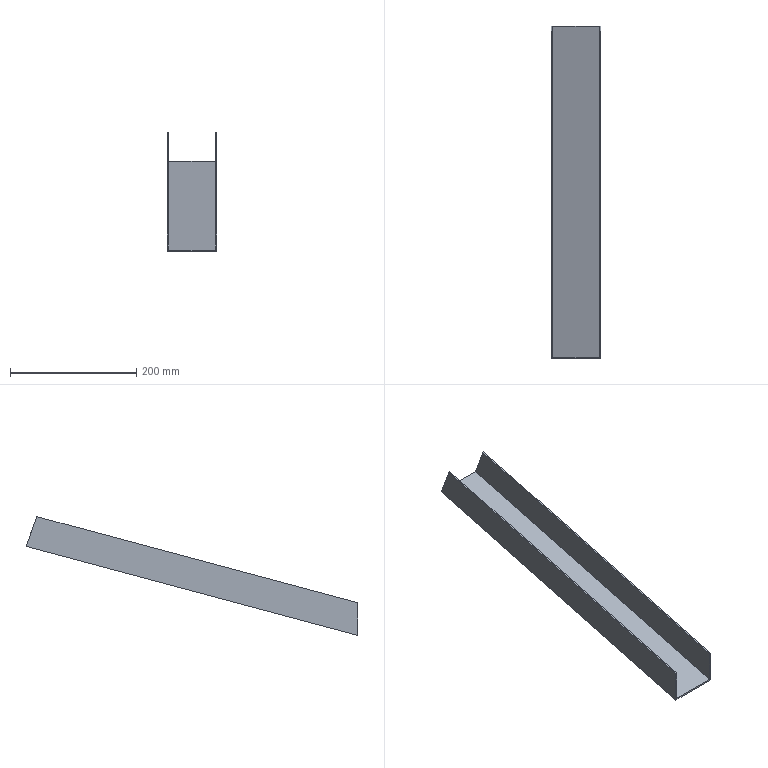Part | NX | features solid 2 | 1 solid | 10 faces | box 78 x 525 x 187.837 mm | volume 187315 mm3 | plane 9 | spline 1
STEP:
#1=CARTESIAN_POINT('',(767.,-915.,-591.646));
#2=VERTEX_POINT('',#1);
#3=CARTESIAN_POINT('',(767.,-407.166,-455.572));
#4=VERTEX_POINT('',#3);
#5=CARTESIAN_POINT('',(767.,-935.325,-597.092));
#6=DIRECTION('',(0.,0.9659,0.2588));
#7=VECTOR('',#6,1000.);
#8=LINE('',#5,#7);
#9=EDGE_CURVE('',#2,#4,#8,.T.);
#10=ORIENTED_EDGE('',*,*,#9,.T.);
#11=CARTESIAN_POINT('',(767.,-390.,-502.736));
#12=VERTEX_POINT('',#11);
#13=CARTESIAN_POINT('',(767.,-407.111,-455.724));
#14=DIRECTION('',(0.,-0.342,0.9397));
#15=VECTOR('',#14,1000.);
#16=LINE('',#13,#15);
#17=EDGE_CURVE('',#12,#4,#16,.T.);
#18=ORIENTED_EDGE('',*,*,#17,.F.);
#19=CARTESIAN_POINT('',(767.,-915.,-643.409));
#20=VERTEX_POINT('',#19);
#21=CARTESIAN_POINT('',(767.,-49.599,-411.526));
#22=DIRECTION('',(0.,0.9659,0.2588));
#23=VECTOR('',#22,1000.);
#24=LINE('',#21,#23);
#25=EDGE_CURVE('',#20,#12,#24,.T.);
#26=ORIENTED_EDGE('',*,*,#25,.F.);
#27=CARTESIAN_POINT('',(767.,-915.,-643.456));
#28=DIRECTION('',(0.,0.,-1.));
#29=VECTOR('',#28,1000.);
#30=LINE('',#27,#29);
#31=EDGE_CURVE('',#2,#20,#30,.T.);
#32=ORIENTED_EDGE('',*,*,#31,.F.);
#33=EDGE_LOOP('',(#10,#18,#26,#32));
#34=FACE_BOUND('',#33,.T.);
#35=CARTESIAN_POINT('',(767.,-922.902,-643.456));
#36=DIRECTION('',(1.,0.,0.));
#37=DIRECTION('',(0.,0.08716,0.9962));
#38=AXIS2_PLACEMENT_3D('',#35,#36,#37);
#39=PLANE('',#38);
#40=ADVANCED_FACE('',(#34),#39,.F.);
#41=CARTESIAN_POINT('',(845.,-915.,-591.646));
#42=VERTEX_POINT('',#41);
#43=CARTESIAN_POINT('',(845.,-915.,-643.409));
#44=VERTEX_POINT('',#43);
#45=CARTESIAN_POINT('',(845.,-915.,-591.646));
#46=CARTESIAN_POINT('',(845.,-915.,-608.9));
#47=CARTESIAN_POINT('',(845.,-915.,-626.155));
#48=CARTESIAN_POINT('',(845.,-915.,-643.409));
#49=B_SPLINE_CURVE_WITH_KNOTS('',3,(#45,#46,#47,#48),.UNSPECIFIED.,.F.,.F.,(4,4),(0.08523,0.137),.UNSPECIFIED.);
#50=EDGE_CURVE('',#42,#44,#49,.T.);
#51=ORIENTED_EDGE('',*,*,#50,.T.);
#52=CARTESIAN_POINT('',(845.,-390.,-502.736));
#53=VERTEX_POINT('',#52);
#54=CARTESIAN_POINT('',(845.,-49.599,-411.526));
#55=DIRECTION('',(0.,0.9659,0.2588));
#56=VECTOR('',#55,1000.);
#57=LINE('',#54,#56);
#58=EDGE_CURVE('',#44,#53,#57,.T.);
#59=ORIENTED_EDGE('',*,*,#58,.T.);
#60=CARTESIAN_POINT('',(845.,-407.166,-455.572));
#61=VERTEX_POINT('',#60);
#62=CARTESIAN_POINT('',(845.,-407.111,-455.724));
#63=DIRECTION('',(0.,-0.342,0.9397));
#64=VECTOR('',#63,1000.);
#65=LINE('',#62,#64);
#66=EDGE_CURVE('',#53,#61,#65,.T.);
#67=ORIENTED_EDGE('',*,*,#66,.T.);
#68=CARTESIAN_POINT('',(845.,-935.325,-597.092));
#69=DIRECTION('',(0.,-0.9659,-0.2588));
#70=VECTOR('',#69,1000.);
#71=LINE('',#68,#70);
#72=EDGE_CURVE('',#42,#61,#71,.F.);
#73=ORIENTED_EDGE('',*,*,#72,.F.);
#74=EDGE_LOOP('',(#51,#59,#67,#73));
#75=FACE_BOUND('',#74,.T.);
#76=CARTESIAN_POINT('',(845.,-922.902,-643.456));
#77=DIRECTION('',(1.,0.,0.));
#78=DIRECTION('',(0.,0.08716,0.9962));
#79=AXIS2_PLACEMENT_3D('',#76,#77,#78);
#80=PLANE('',#79);
#81=ADVANCED_FACE('',(#75),#80,.T.);
#82=CARTESIAN_POINT('',(843.,-390.687,-500.85));
#83=VERTEX_POINT('',#82);
#84=CARTESIAN_POINT('',(843.,-915.,-641.339));
#85=VERTEX_POINT('',#84);
#86=CARTESIAN_POINT('',(843.,-50.117,-409.594));
#87=DIRECTION('',(0.,-0.9659,-0.2588));
#88=VECTOR('',#87,1000.);
#89=LINE('',#86,#88);
#90=EDGE_CURVE('',#83,#85,#89,.T.);
#91=ORIENTED_EDGE('',*,*,#90,.F.);
#92=CARTESIAN_POINT('',(769.,-390.687,-500.85));
#93=VERTEX_POINT('',#92);
#94=CARTESIAN_POINT('',(905.,-390.687,-500.85));
#95=DIRECTION('',(1.,0.,0.));
#96=VECTOR('',#95,1000.);
#97=LINE('',#94,#96);
#98=EDGE_CURVE('',#93,#83,#97,.T.);
#99=ORIENTED_EDGE('',*,*,#98,.F.);
#100=CARTESIAN_POINT('',(769.,-915.,-641.339));
#101=VERTEX_POINT('',#100);
#102=CARTESIAN_POINT('',(769.,-50.117,-409.594));
#103=DIRECTION('',(0.,-0.9659,-0.2588));
#104=VECTOR('',#103,1000.);
#105=LINE('',#102,#104);
#106=EDGE_CURVE('',#93,#101,#105,.T.);
#107=ORIENTED_EDGE('',*,*,#106,.T.);
#108=CARTESIAN_POINT('',(905.,-915.,-641.339));
#109=DIRECTION('',(-1.,0.,0.));
#110=VECTOR('',#109,1000.);
#111=LINE('',#108,#110);
#112=EDGE_CURVE('',#85,#101,#111,.T.);
#113=ORIENTED_EDGE('',*,*,#112,.F.);
#114=EDGE_LOOP('',(#91,#99,#107,#113));
#115=FACE_BOUND('',#114,.T.);
#116=CARTESIAN_POINT('',(905.,-50.117,-409.594));
#117=DIRECTION('',(0.,0.2588,-0.9659));
#118=DIRECTION('',(0.,0.9659,0.2588));
#119=AXIS2_PLACEMENT_3D('',#116,#117,#118);
#120=PLANE('',#119);
#121=ADVANCED_FACE('',(#115),#120,.F.);
#122=CARTESIAN_POINT('',(843.,-915.,-591.646));
#123=VERTEX_POINT('',#122);
#124=CARTESIAN_POINT('',(843.,-915.,-641.339));
#125=CARTESIAN_POINT('',(843.,-915.,-624.774));
#126=CARTESIAN_POINT('',(843.,-915.,-608.21));
#127=CARTESIAN_POINT('',(843.,-915.,-591.646));
#128=B_SPLINE_CURVE_WITH_KNOTS('',3,(#124,#125,#126,#127),.UNSPECIFIED.,.F.,.F.,(4,4),(0.0824,0.1321),.UNSPECIFIED.);
#129=EDGE_CURVE('',#85,#123,#128,.T.);
#130=ORIENTED_EDGE('',*,*,#129,.T.);
#131=CARTESIAN_POINT('',(843.,-407.166,-455.572));
#132=VERTEX_POINT('',#131);
#133=CARTESIAN_POINT('',(843.,-935.325,-597.092));
#134=DIRECTION('',(0.,-0.9659,-0.2588));
#135=VECTOR('',#134,1000.);
#136=LINE('',#133,#135);
#137=EDGE_CURVE('',#123,#132,#136,.F.);
#138=ORIENTED_EDGE('',*,*,#137,.T.);
#139=CARTESIAN_POINT('',(843.,-406.43,-457.596));
#140=DIRECTION('',(0.,0.342,-0.9397));
#141=VECTOR('',#140,1000.);
#142=LINE('',#139,#141);
#143=EDGE_CURVE('',#132,#83,#142,.T.);
#144=ORIENTED_EDGE('',*,*,#143,.T.);
#145=ORIENTED_EDGE('',*,*,#90,.T.);
#146=EDGE_LOOP('',(#130,#138,#144,#145));
#147=FACE_BOUND('',#146,.T.);
#148=CARTESIAN_POINT('',(843.,-922.384,-645.388));
#149=DIRECTION('',(-1.,0.,0.));
#150=DIRECTION('',(0.,-0.08716,-0.9962));
#151=AXIS2_PLACEMENT_3D('',#148,#149,#150);
#152=PLANE('',#151);
#153=ADVANCED_FACE('',(#147),#152,.T.);
#154=CARTESIAN_POINT('',(820.,-915.,-591.646));
#155=DIRECTION('',(-1.,0.,0.));
#156=VECTOR('',#155,1000.);
#157=LINE('',#154,#156);
#158=EDGE_CURVE('',#123,#42,#157,.F.);
#159=ORIENTED_EDGE('',*,*,#158,.T.);
#160=ORIENTED_EDGE('',*,*,#72,.T.);
#161=CARTESIAN_POINT('',(820.,-407.166,-455.572));
#162=DIRECTION('',(1.,0.,0.));
#163=VECTOR('',#162,1000.);
#164=LINE('',#161,#163);
#165=EDGE_CURVE('',#61,#132,#164,.F.);
#166=ORIENTED_EDGE('',*,*,#165,.T.);
#167=ORIENTED_EDGE('',*,*,#137,.F.);
#168=EDGE_LOOP('',(#159,#160,#166,#167));
#169=FACE_BOUND('',#168,.T.);
#170=CARTESIAN_POINT('',(820.,-935.325,-597.092));
#171=DIRECTION('',(0.,0.2588,-0.9659));
#172=DIRECTION('',(0.,0.9659,0.2588));
#173=AXIS2_PLACEMENT_3D('',#170,#171,#172);
#174=PLANE('',#173);
#175=ADVANCED_FACE('',(#169),#174,.F.);
#176=ORIENTED_EDGE('',*,*,#106,.F.);
#177=CARTESIAN_POINT('',(769.,-407.166,-455.572));
#178=VERTEX_POINT('',#177);
#179=CARTESIAN_POINT('',(769.,-406.43,-457.596));
#180=DIRECTION('',(0.,0.342,-0.9397));
#181=VECTOR('',#180,1000.);
#182=LINE('',#179,#181);
#183=EDGE_CURVE('',#178,#93,#182,.T.);
#184=ORIENTED_EDGE('',*,*,#183,.F.);
#185=CARTESIAN_POINT('',(769.,-915.,-591.646));
#186=VERTEX_POINT('',#185);
#187=CARTESIAN_POINT('',(769.,-935.325,-597.092));
#188=DIRECTION('',(0.,0.9659,0.2588));
#189=VECTOR('',#188,1000.);
#190=LINE('',#187,#189);
#191=EDGE_CURVE('',#186,#178,#190,.T.);
#192=ORIENTED_EDGE('',*,*,#191,.F.);
#193=CARTESIAN_POINT('',(769.,-915.,-645.388));
#194=DIRECTION('',(0.,0.,1.));
#195=VECTOR('',#194,1000.);
#196=LINE('',#193,#195);
#197=EDGE_CURVE('',#101,#186,#196,.T.);
#198=ORIENTED_EDGE('',*,*,#197,.F.);
#199=EDGE_LOOP('',(#176,#184,#192,#198));
#200=FACE_BOUND('',#199,.T.);
#201=CARTESIAN_POINT('',(769.,-922.384,-645.388));
#202=DIRECTION('',(-1.,0.,0.));
#203=DIRECTION('',(0.,-0.08716,-0.9962));
#204=AXIS2_PLACEMENT_3D('',#201,#202,#203);
#205=PLANE('',#204);
#206=ADVANCED_FACE('',(#200),#205,.F.);
#207=ORIENTED_EDGE('',*,*,#191,.T.);
#208=CARTESIAN_POINT('',(750.,-407.166,-455.572));
#209=DIRECTION('',(1.,0.,0.));
#210=VECTOR('',#209,1000.);
#211=LINE('',#208,#210);
#212=EDGE_CURVE('',#4,#178,#211,.T.);
#213=ORIENTED_EDGE('',*,*,#212,.F.);
#214=ORIENTED_EDGE('',*,*,#9,.F.);
#215=CARTESIAN_POINT('',(750.,-915.,-591.646));
#216=DIRECTION('',(-1.,0.,0.));
#217=VECTOR('',#216,1000.);
#218=LINE('',#215,#217);
#219=EDGE_CURVE('',#186,#2,#218,.T.);
#220=ORIENTED_EDGE('',*,*,#219,.F.);
#221=EDGE_LOOP('',(#207,#213,#214,#220));
#222=FACE_BOUND('',#221,.T.);
#223=CARTESIAN_POINT('',(750.,-935.325,-597.092));
#224=DIRECTION('',(0.,0.2588,-0.9659));
#225=DIRECTION('',(0.,0.9659,0.2588));
#226=AXIS2_PLACEMENT_3D('',#223,#224,#225);
#227=PLANE('',#226);
#228=ADVANCED_FACE('',(#222),#227,.F.);
#229=CARTESIAN_POINT('',(905.,-915.,-643.409));
#230=DIRECTION('',(-1.,0.,0.));
#231=VECTOR('',#230,1000.);
#232=LINE('',#229,#231);
#233=EDGE_CURVE('',#44,#20,#232,.T.);
#234=ORIENTED_EDGE('',*,*,#233,.T.);
#235=ORIENTED_EDGE('',*,*,#25,.T.);
#236=CARTESIAN_POINT('',(905.,-390.,-502.736));
#237=DIRECTION('',(-1.,0.,0.));
#238=VECTOR('',#237,1000.);
#239=LINE('',#236,#238);
#240=EDGE_CURVE('',#53,#12,#239,.T.);
#241=ORIENTED_EDGE('',*,*,#240,.F.);
#242=ORIENTED_EDGE('',*,*,#58,.F.);
#243=EDGE_LOOP('',(#234,#235,#241,#242));
#244=FACE_BOUND('',#243,.T.);
#245=CARTESIAN_POINT('',(905.,-49.599,-411.526));
#246=DIRECTION('',(0.,0.2588,-0.9659));
#247=DIRECTION('',(0.,0.9659,0.2588));
#248=AXIS2_PLACEMENT_3D('',#245,#246,#247);
#249=PLANE('',#248);
#250=ADVANCED_FACE('',(#244),#249,.T.);
#251=ORIENTED_EDGE('',*,*,#98,.T.);
#252=ORIENTED_EDGE('',*,*,#143,.F.);
#253=ORIENTED_EDGE('',*,*,#165,.F.);
#254=ORIENTED_EDGE('',*,*,#66,.F.);
#255=ORIENTED_EDGE('',*,*,#240,.T.);
#256=ORIENTED_EDGE('',*,*,#17,.T.);
#257=ORIENTED_EDGE('',*,*,#212,.T.);
#258=ORIENTED_EDGE('',*,*,#183,.T.);
#259=EDGE_LOOP('',(#251,#252,#253,#254,#255,#256,#257,#258));
#260=FACE_BOUND('',#259,.T.);
#261=CARTESIAN_POINT('',(825.,-390.,-502.736));
#262=DIRECTION('',(0.,-0.9397,-0.342));
#263=DIRECTION('',(0.,0.342,-0.9397));
#264=AXIS2_PLACEMENT_3D('',#261,#262,#263);
#265=PLANE('',#264);
#266=ADVANCED_FACE('',(#260),#265,.F.);
#267=ORIENTED_EDGE('',*,*,#112,.T.);
#268=ORIENTED_EDGE('',*,*,#197,.T.);
#269=ORIENTED_EDGE('',*,*,#219,.T.);
#270=ORIENTED_EDGE('',*,*,#31,.T.);
#271=ORIENTED_EDGE('',*,*,#233,.F.);
#272=ORIENTED_EDGE('',*,*,#50,.F.);
#273=ORIENTED_EDGE('',*,*,#158,.F.);
#274=ORIENTED_EDGE('',*,*,#129,.F.);
#275=EDGE_LOOP('',(#267,#268,#269,#270,#271,#272,#273,#274));
#276=FACE_BOUND('',#275,.T.);
#277=CARTESIAN_POINT('',(767.,-915.,-643.409));
#278=CARTESIAN_POINT('',(767.,-915.,-591.646));
#279=CARTESIAN_POINT('',(845.,-915.,-643.409));
#280=CARTESIAN_POINT('',(845.,-915.,-591.646));
#281=B_SPLINE_SURFACE_WITH_KNOTS('',1,1,((#277,#278),(#279,#280)),.PLANE_SURF.,.F.,.F.,.F.,(2,2),(2,2),(0.442,0.5062),(0.68,0.7846),.PIECEWISE_BEZIER_KNOTS.);
#282=ADVANCED_FACE('',(#276),#281,.T.);
#283=CLOSED_SHELL('',(#40,#81,#121,#153,#175,#206,#228,#250,#266,#282));
#284=MANIFOLD_SOLID_BREP('',#283);
#285=(LENGTH_UNIT()NAMED_UNIT(*)SI_UNIT(.MILLI.,.METRE.));
#286=UNCERTAINTY_MEASURE_WITH_UNIT(LENGTH_MEASURE(0.0508),#285,'','');
#287=(NAMED_UNIT(*)PLANE_ANGLE_UNIT()SI_UNIT($,.RADIAN.));
#288=(NAMED_UNIT(*)SI_UNIT($,.STERADIAN.)SOLID_ANGLE_UNIT());
#289=(GEOMETRIC_REPRESENTATION_CONTEXT(3)GLOBAL_UNCERTAINTY_ASSIGNED_CONTEXT((#286))GLOBAL_UNIT_ASSIGNED_CONTEXT((#285,#287,#288))REPRESENTATION_CONTEXT('',''));
#290=ADVANCED_BREP_SHAPE_REPRESENTATION('',(#284),#289);